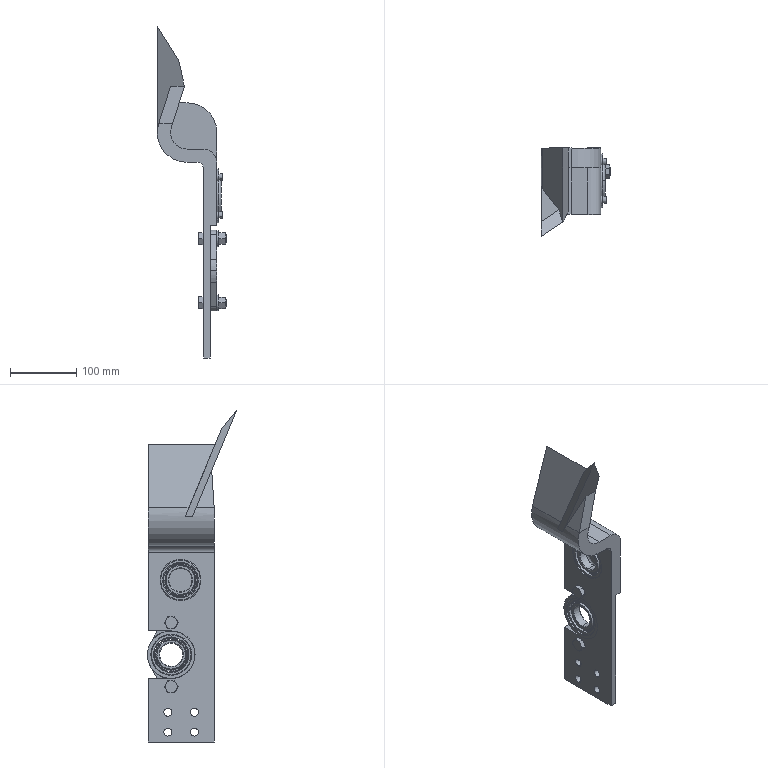Part | SolidWorks | 15 solids | 1100 faces | box 105 x 134.847 x 502.101 mm | volume 896444 mm3 | cone 378 | cylinder 245 | plane 189 | sphere 176 | torus 112 | commonest cylinder face diameters 6 x128 12 x24 62 x10 5 x8 10 x8 43.3 x8